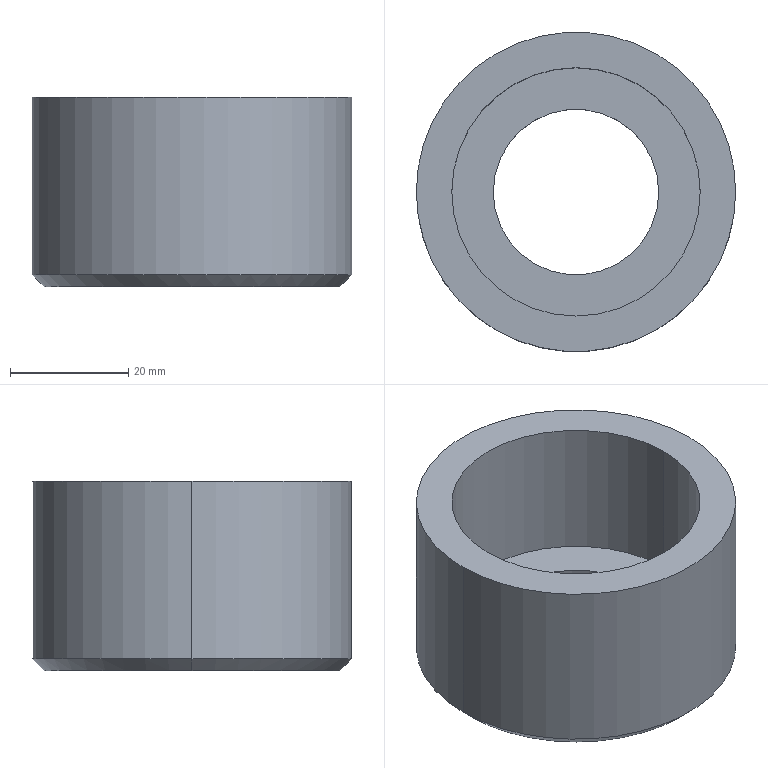Part | SolidWorks | features Chamfer 1, Extrusion 1, ICE 1 | 1 solid | 11 faces | box 54 x 54 x 32 mm | volume 34780 mm3 | cylinder 6 | plane 3 | cone 2 | commonest cylinder face diameters 28 x2 42 x2 54 x2
STEP:
#1=CARTESIAN_POINT('',(-25.,0.,0.));
#2=VERTEX_POINT('',#1);
#3=CARTESIAN_POINT('',(25.,0.,0.));
#4=VERTEX_POINT('',#3);
#5=CARTESIAN_POINT('',(0.,0.,0.));
#6=DIRECTION('',(0.,0.,-1.));
#7=DIRECTION('',(1.,0.,0.));
#8=AXIS2_PLACEMENT_3D('',#5,#6,#7);
#9=CIRCLE('',#8,25.);
#10=EDGE_CURVE('',#2,#4,#9,.T.);
#11=ORIENTED_EDGE('',*,*,#10,.F.);
#12=CARTESIAN_POINT('',(-27.,0.,2.));
#13=VERTEX_POINT('',#12);
#14=CARTESIAN_POINT('',(-27.,0.,2.));
#15=DIRECTION('',(-0.7071,0.,0.7071));
#16=VECTOR('',#15,1000.);
#17=LINE('',#14,#16);
#18=EDGE_CURVE('',#2,#13,#17,.T.);
#19=ORIENTED_EDGE('',*,*,#18,.T.);
#20=CARTESIAN_POINT('',(27.,0.,2.));
#21=VERTEX_POINT('',#20);
#22=CARTESIAN_POINT('',(0.,0.,2.));
#23=DIRECTION('',(0.,0.,1.));
#24=DIRECTION('',(1.,0.,0.));
#25=AXIS2_PLACEMENT_3D('',#22,#23,#24);
#26=CIRCLE('',#25,27.);
#27=EDGE_CURVE('',#21,#13,#26,.T.);
#28=ORIENTED_EDGE('',*,*,#27,.F.);
#29=CARTESIAN_POINT('',(27.,0.,2.));
#30=DIRECTION('',(0.7071,0.,0.7071));
#31=VECTOR('',#30,1000.);
#32=LINE('',#29,#31);
#33=EDGE_CURVE('',#4,#21,#32,.T.);
#34=ORIENTED_EDGE('',*,*,#33,.F.);
#35=EDGE_LOOP('',(#11,#19,#28,#34));
#36=FACE_OUTER_BOUND('',#35,.T.);
#37=CARTESIAN_POINT('',(0.,0.,2.));
#38=DIRECTION('',(0.,0.,1.));
#39=DIRECTION('',(1.,0.,0.));
#40=AXIS2_PLACEMENT_3D('',#37,#38,#39);
#41=CONICAL_SURFACE('',#40,27.,0.7854);
#42=ADVANCED_FACE('',(#36),#41,.T.);
#43=CARTESIAN_POINT('',(-21.,0.,8.));
#44=VERTEX_POINT('',#43);
#45=CARTESIAN_POINT('',(21.,0.,8.));
#46=VERTEX_POINT('',#45);
#47=CARTESIAN_POINT('',(0.,0.,8.));
#48=DIRECTION('',(0.,0.,1.));
#49=DIRECTION('',(1.,0.,0.));
#50=AXIS2_PLACEMENT_3D('',#47,#48,#49);
#51=CIRCLE('',#50,21.);
#52=EDGE_CURVE('',#44,#46,#51,.T.);
#53=ORIENTED_EDGE('',*,*,#52,.F.);
#54=CARTESIAN_POINT('',(-21.,0.,32.));
#55=VERTEX_POINT('',#54);
#56=CARTESIAN_POINT('',(-21.,0.,8.));
#57=DIRECTION('',(0.,0.,1.));
#58=VECTOR('',#57,1000.);
#59=LINE('',#56,#58);
#60=EDGE_CURVE('',#44,#55,#59,.T.);
#61=ORIENTED_EDGE('',*,*,#60,.T.);
#62=CARTESIAN_POINT('',(21.,0.,32.));
#63=VERTEX_POINT('',#62);
#64=CARTESIAN_POINT('',(0.,0.,32.));
#65=DIRECTION('',(0.,0.,1.));
#66=DIRECTION('',(1.,0.,0.));
#67=AXIS2_PLACEMENT_3D('',#64,#65,#66);
#68=CIRCLE('',#67,21.);
#69=EDGE_CURVE('',#55,#63,#68,.T.);
#70=ORIENTED_EDGE('',*,*,#69,.T.);
#71=CARTESIAN_POINT('',(21.,0.,8.));
#72=DIRECTION('',(0.,0.,1.));
#73=VECTOR('',#72,1000.);
#74=LINE('',#71,#73);
#75=EDGE_CURVE('',#46,#63,#74,.T.);
#76=ORIENTED_EDGE('',*,*,#75,.F.);
#77=EDGE_LOOP('',(#53,#61,#70,#76));
#78=FACE_OUTER_BOUND('',#77,.T.);
#79=CARTESIAN_POINT('',(0.,0.,8.));
#80=DIRECTION('',(0.,0.,1.));
#81=DIRECTION('',(1.,0.,0.));
#82=AXIS2_PLACEMENT_3D('',#79,#80,#81);
#83=CYLINDRICAL_SURFACE('',#82,21.);
#84=ADVANCED_FACE('',(#78),#83,.F.);
#85=CARTESIAN_POINT('',(27.,0.,32.));
#86=VERTEX_POINT('',#85);
#87=CARTESIAN_POINT('',(-27.,0.,32.));
#88=VERTEX_POINT('',#87);
#89=CARTESIAN_POINT('',(0.,0.,32.));
#90=DIRECTION('',(0.,0.,1.));
#91=DIRECTION('',(1.,0.,0.));
#92=AXIS2_PLACEMENT_3D('',#89,#90,#91);
#93=CIRCLE('',#92,27.);
#94=EDGE_CURVE('',#86,#88,#93,.T.);
#95=ORIENTED_EDGE('',*,*,#94,.F.);
#96=CARTESIAN_POINT('',(27.,0.,32.));
#97=DIRECTION('',(0.,0.,-1.));
#98=VECTOR('',#97,1000.);
#99=LINE('',#96,#98);
#100=EDGE_CURVE('',#86,#21,#99,.T.);
#101=ORIENTED_EDGE('',*,*,#100,.T.);
#102=ORIENTED_EDGE('',*,*,#27,.T.);
#103=CARTESIAN_POINT('',(-27.,0.,32.));
#104=DIRECTION('',(0.,0.,-1.));
#105=VECTOR('',#104,1000.);
#106=LINE('',#103,#105);
#107=EDGE_CURVE('',#88,#13,#106,.T.);
#108=ORIENTED_EDGE('',*,*,#107,.F.);
#109=EDGE_LOOP('',(#95,#101,#102,#108));
#110=FACE_OUTER_BOUND('',#109,.T.);
#111=CARTESIAN_POINT('',(0.,0.,32.));
#112=DIRECTION('',(0.,0.,-1.));
#113=DIRECTION('',(-1.,0.,0.));
#114=AXIS2_PLACEMENT_3D('',#111,#112,#113);
#115=CYLINDRICAL_SURFACE('',#114,27.);
#116=ADVANCED_FACE('',(#110),#115,.T.);
#117=CARTESIAN_POINT('',(-14.,0.,8.));
#118=VERTEX_POINT('',#117);
#119=CARTESIAN_POINT('',(14.,0.,8.));
#120=VERTEX_POINT('',#119);
#121=CARTESIAN_POINT('',(0.,0.,8.));
#122=DIRECTION('',(0.,0.,1.));
#123=DIRECTION('',(1.,0.,0.));
#124=AXIS2_PLACEMENT_3D('',#121,#122,#123);
#125=CIRCLE('',#124,14.);
#126=EDGE_CURVE('',#118,#120,#125,.T.);
#127=ORIENTED_EDGE('',*,*,#126,.T.);
#128=CARTESIAN_POINT('',(14.,0.,0.));
#129=VERTEX_POINT('',#128);
#130=CARTESIAN_POINT('',(14.,0.,32.));
#131=DIRECTION('',(0.,0.,-1.));
#132=VECTOR('',#131,1000.);
#133=LINE('',#130,#132);
#134=EDGE_CURVE('',#120,#129,#133,.T.);
#135=ORIENTED_EDGE('',*,*,#134,.T.);
#136=CARTESIAN_POINT('',(-14.,0.,0.));
#137=VERTEX_POINT('',#136);
#138=CARTESIAN_POINT('',(0.,0.,0.));
#139=DIRECTION('',(0.,0.,1.));
#140=DIRECTION('',(1.,0.,0.));
#141=AXIS2_PLACEMENT_3D('',#138,#139,#140);
#142=CIRCLE('',#141,14.);
#143=EDGE_CURVE('',#137,#129,#142,.T.);
#144=ORIENTED_EDGE('',*,*,#143,.F.);
#145=CARTESIAN_POINT('',(-14.,0.,32.));
#146=DIRECTION('',(0.,0.,-1.));
#147=VECTOR('',#146,1000.);
#148=LINE('',#145,#147);
#149=EDGE_CURVE('',#118,#137,#148,.T.);
#150=ORIENTED_EDGE('',*,*,#149,.F.);
#151=EDGE_LOOP('',(#127,#135,#144,#150));
#152=FACE_OUTER_BOUND('',#151,.T.);
#153=CARTESIAN_POINT('',(0.,0.,32.));
#154=DIRECTION('',(0.,0.,-1.));
#155=DIRECTION('',(-1.,0.,0.));
#156=AXIS2_PLACEMENT_3D('',#153,#154,#155);
#157=CYLINDRICAL_SURFACE('',#156,14.);
#158=ADVANCED_FACE('',(#152),#157,.F.);
#159=ORIENTED_EDGE('',*,*,#134,.F.);
#160=CARTESIAN_POINT('',(0.,0.,8.));
#161=DIRECTION('',(0.,0.,1.));
#162=DIRECTION('',(1.,0.,0.));
#163=AXIS2_PLACEMENT_3D('',#160,#161,#162);
#164=CIRCLE('',#163,14.);
#165=EDGE_CURVE('',#120,#118,#164,.T.);
#166=ORIENTED_EDGE('',*,*,#165,.T.);
#167=ORIENTED_EDGE('',*,*,#149,.T.);
#168=CARTESIAN_POINT('',(0.,0.,0.));
#169=DIRECTION('',(0.,0.,1.));
#170=DIRECTION('',(1.,0.,0.));
#171=AXIS2_PLACEMENT_3D('',#168,#169,#170);
#172=CIRCLE('',#171,14.);
#173=EDGE_CURVE('',#129,#137,#172,.T.);
#174=ORIENTED_EDGE('',*,*,#173,.F.);
#175=EDGE_LOOP('',(#159,#166,#167,#174));
#176=FACE_OUTER_BOUND('',#175,.T.);
#177=CARTESIAN_POINT('',(0.,0.,32.));
#178=DIRECTION('',(0.,0.,-1.));
#179=DIRECTION('',(-1.,0.,0.));
#180=AXIS2_PLACEMENT_3D('',#177,#178,#179);
#181=CYLINDRICAL_SURFACE('',#180,14.);
#182=ADVANCED_FACE('',(#176),#181,.F.);
#183=CARTESIAN_POINT('',(0.,0.,32.));
#184=DIRECTION('',(0.,0.,1.));
#185=DIRECTION('',(1.,0.,0.));
#186=AXIS2_PLACEMENT_3D('',#183,#184,#185);
#187=CIRCLE('',#186,21.);
#188=EDGE_CURVE('',#63,#55,#187,.T.);
#189=ORIENTED_EDGE('',*,*,#188,.F.);
#190=ORIENTED_EDGE('',*,*,#69,.F.);
#191=EDGE_LOOP('',(#189,#190));
#192=FACE_BOUND('',#191,.T.);
#193=CARTESIAN_POINT('',(0.,0.,32.));
#194=DIRECTION('',(0.,0.,1.));
#195=DIRECTION('',(1.,0.,0.));
#196=AXIS2_PLACEMENT_3D('',#193,#194,#195);
#197=CIRCLE('',#196,27.);
#198=EDGE_CURVE('',#88,#86,#197,.T.);
#199=ORIENTED_EDGE('',*,*,#198,.T.);
#200=ORIENTED_EDGE('',*,*,#94,.T.);
#201=EDGE_LOOP('',(#199,#200));
#202=FACE_OUTER_BOUND('',#201,.T.);
#203=CARTESIAN_POINT('',(0.,0.,32.));
#204=DIRECTION('',(0.,0.,1.));
#205=DIRECTION('',(1.,0.,0.));
#206=AXIS2_PLACEMENT_3D('',#203,#204,#205);
#207=PLANE('',#206);
#208=ADVANCED_FACE('',(#192,#202),#207,.T.);
#209=CARTESIAN_POINT('',(0.,0.,0.));
#210=DIRECTION('',(0.,0.,-1.));
#211=DIRECTION('',(1.,0.,0.));
#212=AXIS2_PLACEMENT_3D('',#209,#210,#211);
#213=CIRCLE('',#212,25.);
#214=EDGE_CURVE('',#4,#2,#213,.T.);
#215=ORIENTED_EDGE('',*,*,#214,.T.);
#216=ORIENTED_EDGE('',*,*,#10,.T.);
#217=EDGE_LOOP('',(#215,#216));
#218=FACE_OUTER_BOUND('',#217,.T.);
#219=ORIENTED_EDGE('',*,*,#143,.T.);
#220=ORIENTED_EDGE('',*,*,#173,.T.);
#221=EDGE_LOOP('',(#219,#220));
#222=FACE_BOUND('',#221,.T.);
#223=CARTESIAN_POINT('',(0.,0.,0.));
#224=DIRECTION('',(0.,0.,1.));
#225=DIRECTION('',(1.,0.,0.));
#226=AXIS2_PLACEMENT_3D('',#223,#224,#225);
#227=PLANE('',#226);
#228=ADVANCED_FACE('',(#218,#222),#227,.F.);
#229=ORIENTED_EDGE('',*,*,#100,.F.);
#230=ORIENTED_EDGE('',*,*,#198,.F.);
#231=ORIENTED_EDGE('',*,*,#107,.T.);
#232=CARTESIAN_POINT('',(0.,0.,2.));
#233=DIRECTION('',(0.,0.,1.));
#234=DIRECTION('',(1.,0.,0.));
#235=AXIS2_PLACEMENT_3D('',#232,#233,#234);
#236=CIRCLE('',#235,27.);
#237=EDGE_CURVE('',#13,#21,#236,.T.);
#238=ORIENTED_EDGE('',*,*,#237,.T.);
#239=EDGE_LOOP('',(#229,#230,#231,#238));
#240=FACE_OUTER_BOUND('',#239,.T.);
#241=CARTESIAN_POINT('',(0.,0.,32.));
#242=DIRECTION('',(0.,0.,-1.));
#243=DIRECTION('',(-1.,0.,0.));
#244=AXIS2_PLACEMENT_3D('',#241,#242,#243);
#245=CYLINDRICAL_SURFACE('',#244,27.);
#246=ADVANCED_FACE('',(#240),#245,.T.);
#247=ORIENTED_EDGE('',*,*,#60,.F.);
#248=CARTESIAN_POINT('',(0.,0.,8.));
#249=DIRECTION('',(0.,0.,1.));
#250=DIRECTION('',(1.,0.,0.));
#251=AXIS2_PLACEMENT_3D('',#248,#249,#250);
#252=CIRCLE('',#251,21.);
#253=EDGE_CURVE('',#46,#44,#252,.T.);
#254=ORIENTED_EDGE('',*,*,#253,.F.);
#255=ORIENTED_EDGE('',*,*,#75,.T.);
#256=ORIENTED_EDGE('',*,*,#188,.T.);
#257=EDGE_LOOP('',(#247,#254,#255,#256));
#258=FACE_OUTER_BOUND('',#257,.T.);
#259=CARTESIAN_POINT('',(0.,0.,8.));
#260=DIRECTION('',(0.,0.,1.));
#261=DIRECTION('',(1.,0.,0.));
#262=AXIS2_PLACEMENT_3D('',#259,#260,#261);
#263=CYLINDRICAL_SURFACE('',#262,21.);
#264=ADVANCED_FACE('',(#258),#263,.F.);
#265=ORIENTED_EDGE('',*,*,#126,.F.);
#266=ORIENTED_EDGE('',*,*,#165,.F.);
#267=EDGE_LOOP('',(#265,#266));
#268=FACE_BOUND('',#267,.T.);
#269=ORIENTED_EDGE('',*,*,#253,.T.);
#270=ORIENTED_EDGE('',*,*,#52,.T.);
#271=EDGE_LOOP('',(#269,#270));
#272=FACE_OUTER_BOUND('',#271,.T.);
#273=CARTESIAN_POINT('',(0.,0.,8.));
#274=DIRECTION('',(0.,0.,1.));
#275=DIRECTION('',(1.,0.,0.));
#276=AXIS2_PLACEMENT_3D('',#273,#274,#275);
#277=PLANE('',#276);
#278=ADVANCED_FACE('',(#268,#272),#277,.T.);
#279=ORIENTED_EDGE('',*,*,#18,.F.);
#280=ORIENTED_EDGE('',*,*,#214,.F.);
#281=ORIENTED_EDGE('',*,*,#33,.T.);
#282=ORIENTED_EDGE('',*,*,#237,.F.);
#283=EDGE_LOOP('',(#279,#280,#281,#282));
#284=FACE_OUTER_BOUND('',#283,.T.);
#285=CARTESIAN_POINT('',(0.,0.,2.));
#286=DIRECTION('',(0.,0.,1.));
#287=DIRECTION('',(1.,0.,0.));
#288=AXIS2_PLACEMENT_3D('',#285,#286,#287);
#289=CONICAL_SURFACE('',#288,27.,0.7854);
#290=ADVANCED_FACE('',(#284),#289,.T.);
#291=CLOSED_SHELL('',(#42,#84,#116,#158,#182,#208,#228,#246,#264,#278,#290));
#292=MANIFOLD_SOLID_BREP('',#291);
#293=CARTESIAN_POINT('',(0.,0.,0.));
#294=DIRECTION('',(0.,0.,1.));
#295=DIRECTION('',(1.,0.,0.));
#296=AXIS2_PLACEMENT_3D('',#293,#294,#295);
#297=(LENGTH_UNIT()NAMED_UNIT(*)SI_UNIT(.MILLI.,.METRE.));
#298=UNCERTAINTY_MEASURE_WITH_UNIT(LENGTH_MEASURE(0.00001),#297,'','');
#299=(NAMED_UNIT(*)PLANE_ANGLE_UNIT()SI_UNIT($,.RADIAN.));
#300=(NAMED_UNIT(*)SI_UNIT($,.STERADIAN.)SOLID_ANGLE_UNIT());
#301=(GEOMETRIC_REPRESENTATION_CONTEXT(3)GLOBAL_UNCERTAINTY_ASSIGNED_CONTEXT((#298))GLOBAL_UNIT_ASSIGNED_CONTEXT((#297,#299,#300))REPRESENTATION_CONTEXT('',''));
#302=ADVANCED_BREP_SHAPE_REPRESENTATION('',(#292,#296),#301);